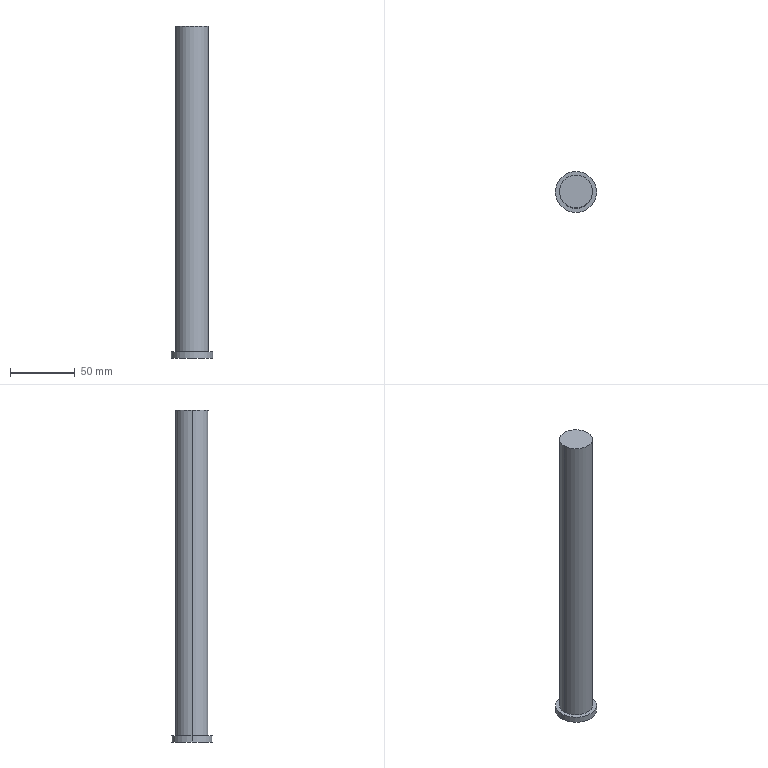Part | STEP file | 4-20.sldasm-Part-242 | 1 solid | 7 faces | box 31.75 x 31.75 x 256 mm | volume 131075 mm3 | cylinder 4 | plane 3 | commonest cylinder face diameters 25.4 x2 31.75 x2
STEP:
#1=CARTESIAN_POINT('',(105.7,-492.,-100.237));
#2=VERTEX_POINT('',#1);
#3=CARTESIAN_POINT('',(80.3,-492.,-100.237));
#4=VERTEX_POINT('',#3);
#5=CARTESIAN_POINT('',(93.,-492.,-100.237));
#6=DIRECTION('',(0.,0.,-1.));
#7=DIRECTION('',(1.,0.,0.));
#8=AXIS2_PLACEMENT_3D('',#5,#6,#7);
#9=CIRCLE('',#8,12.7);
#10=EDGE_CURVE('',#2,#4,#9,.T.);
#11=ORIENTED_EDGE('',*,*,#10,.F.);
#12=CARTESIAN_POINT('',(105.7,-492.,151.));
#13=VERTEX_POINT('',#12);
#14=CARTESIAN_POINT('',(105.7,-492.,93.299));
#15=DIRECTION('',(0.,0.,1.));
#16=VECTOR('',#15,1000.);
#17=LINE('',#14,#16);
#18=EDGE_CURVE('',#2,#13,#17,.T.);
#19=ORIENTED_EDGE('',*,*,#18,.T.);
#20=CARTESIAN_POINT('',(80.3,-492.,151.));
#21=VERTEX_POINT('',#20);
#22=CARTESIAN_POINT('',(93.,-492.,151.));
#23=DIRECTION('',(0.,0.,-1.));
#24=DIRECTION('',(1.,0.,0.));
#25=AXIS2_PLACEMENT_3D('',#22,#23,#24);
#26=CIRCLE('',#25,12.7);
#27=EDGE_CURVE('',#13,#21,#26,.T.);
#28=ORIENTED_EDGE('',*,*,#27,.T.);
#29=CARTESIAN_POINT('',(80.3,-492.,93.299));
#30=DIRECTION('',(0.,0.,1.));
#31=VECTOR('',#30,1000.);
#32=LINE('',#29,#31);
#33=EDGE_CURVE('',#4,#21,#32,.T.);
#34=ORIENTED_EDGE('',*,*,#33,.F.);
#35=EDGE_LOOP('',(#11,#19,#28,#34));
#36=FACE_OUTER_BOUND('',#35,.T.);
#37=CARTESIAN_POINT('',(93.,-492.,93.299));
#38=DIRECTION('',(0.,0.,1.));
#39=DIRECTION('',(-1.,0.,0.));
#40=AXIS2_PLACEMENT_3D('',#37,#38,#39);
#41=CYLINDRICAL_SURFACE('',#40,12.7);
#42=ADVANCED_FACE('',(#36),#41,.T.);
#43=CARTESIAN_POINT('',(108.875,-492.,-105.));
#44=VERTEX_POINT('',#43);
#45=CARTESIAN_POINT('',(77.125,-492.,-105.));
#46=VERTEX_POINT('',#45);
#47=CARTESIAN_POINT('',(93.,-492.,-105.));
#48=DIRECTION('',(0.,0.,-1.));
#49=DIRECTION('',(1.,0.,0.));
#50=AXIS2_PLACEMENT_3D('',#47,#48,#49);
#51=CIRCLE('',#50,15.875);
#52=EDGE_CURVE('',#44,#46,#51,.T.);
#53=ORIENTED_EDGE('',*,*,#52,.F.);
#54=CARTESIAN_POINT('',(108.875,-492.,-100.237));
#55=VERTEX_POINT('',#54);
#56=CARTESIAN_POINT('',(108.875,-492.,93.299));
#57=DIRECTION('',(0.,0.,1.));
#58=VECTOR('',#57,1000.);
#59=LINE('',#56,#58);
#60=EDGE_CURVE('',#44,#55,#59,.T.);
#61=ORIENTED_EDGE('',*,*,#60,.T.);
#62=CARTESIAN_POINT('',(77.125,-492.,-100.237));
#63=VERTEX_POINT('',#62);
#64=CARTESIAN_POINT('',(93.,-492.,-100.237));
#65=DIRECTION('',(0.,0.,-1.));
#66=DIRECTION('',(1.,0.,0.));
#67=AXIS2_PLACEMENT_3D('',#64,#65,#66);
#68=CIRCLE('',#67,15.875);
#69=EDGE_CURVE('',#55,#63,#68,.T.);
#70=ORIENTED_EDGE('',*,*,#69,.T.);
#71=CARTESIAN_POINT('',(77.125,-492.,93.299));
#72=DIRECTION('',(0.,0.,1.));
#73=VECTOR('',#72,1000.);
#74=LINE('',#71,#73);
#75=EDGE_CURVE('',#46,#63,#74,.T.);
#76=ORIENTED_EDGE('',*,*,#75,.F.);
#77=EDGE_LOOP('',(#53,#61,#70,#76));
#78=FACE_OUTER_BOUND('',#77,.T.);
#79=CARTESIAN_POINT('',(93.,-492.,93.299));
#80=DIRECTION('',(0.,0.,1.));
#81=DIRECTION('',(-1.,0.,0.));
#82=AXIS2_PLACEMENT_3D('',#79,#80,#81);
#83=CYLINDRICAL_SURFACE('',#82,15.875);
#84=ADVANCED_FACE('',(#78),#83,.T.);
#85=CARTESIAN_POINT('',(93.,-492.,-100.237));
#86=DIRECTION('',(0.,0.,-1.));
#87=DIRECTION('',(1.,0.,0.));
#88=AXIS2_PLACEMENT_3D('',#85,#86,#87);
#89=CIRCLE('',#88,12.7);
#90=EDGE_CURVE('',#4,#2,#89,.T.);
#91=ORIENTED_EDGE('',*,*,#90,.T.);
#92=ORIENTED_EDGE('',*,*,#10,.T.);
#93=EDGE_LOOP('',(#91,#92));
#94=FACE_BOUND('',#93,.T.);
#95=CARTESIAN_POINT('',(93.,-492.,-100.237));
#96=DIRECTION('',(0.,0.,-1.));
#97=DIRECTION('',(1.,0.,0.));
#98=AXIS2_PLACEMENT_3D('',#95,#96,#97);
#99=CIRCLE('',#98,15.875);
#100=EDGE_CURVE('',#63,#55,#99,.T.);
#101=ORIENTED_EDGE('',*,*,#100,.F.);
#102=ORIENTED_EDGE('',*,*,#69,.F.);
#103=EDGE_LOOP('',(#101,#102));
#104=FACE_OUTER_BOUND('',#103,.T.);
#105=CARTESIAN_POINT('',(93.,-492.,-100.237));
#106=DIRECTION('',(0.,0.,1.));
#107=DIRECTION('',(-1.,0.,0.));
#108=AXIS2_PLACEMENT_3D('',#105,#106,#107);
#109=PLANE('',#108);
#110=ADVANCED_FACE('',(#94,#104),#109,.T.);
#111=CARTESIAN_POINT('',(93.,-492.,-105.));
#112=DIRECTION('',(0.,0.,-1.));
#113=DIRECTION('',(1.,0.,0.));
#114=AXIS2_PLACEMENT_3D('',#111,#112,#113);
#115=CIRCLE('',#114,15.875);
#116=EDGE_CURVE('',#46,#44,#115,.T.);
#117=ORIENTED_EDGE('',*,*,#116,.T.);
#118=ORIENTED_EDGE('',*,*,#52,.T.);
#119=EDGE_LOOP('',(#117,#118));
#120=FACE_OUTER_BOUND('',#119,.T.);
#121=CARTESIAN_POINT('',(93.,-492.,-105.));
#122=DIRECTION('',(0.,0.,1.));
#123=DIRECTION('',(-1.,0.,0.));
#124=AXIS2_PLACEMENT_3D('',#121,#122,#123);
#125=PLANE('',#124);
#126=ADVANCED_FACE('',(#120),#125,.F.);
#127=ORIENTED_EDGE('',*,*,#60,.F.);
#128=ORIENTED_EDGE('',*,*,#116,.F.);
#129=ORIENTED_EDGE('',*,*,#75,.T.);
#130=ORIENTED_EDGE('',*,*,#100,.T.);
#131=EDGE_LOOP('',(#127,#128,#129,#130));
#132=FACE_OUTER_BOUND('',#131,.T.);
#133=CARTESIAN_POINT('',(93.,-492.,93.299));
#134=DIRECTION('',(0.,0.,1.));
#135=DIRECTION('',(-1.,0.,0.));
#136=AXIS2_PLACEMENT_3D('',#133,#134,#135);
#137=CYLINDRICAL_SURFACE('',#136,15.875);
#138=ADVANCED_FACE('',(#132),#137,.T.);
#139=CARTESIAN_POINT('',(93.,-492.,151.));
#140=DIRECTION('',(0.,0.,-1.));
#141=DIRECTION('',(1.,0.,0.));
#142=AXIS2_PLACEMENT_3D('',#139,#140,#141);
#143=CIRCLE('',#142,12.7);
#144=EDGE_CURVE('',#21,#13,#143,.T.);
#145=ORIENTED_EDGE('',*,*,#144,.F.);
#146=ORIENTED_EDGE('',*,*,#27,.F.);
#147=EDGE_LOOP('',(#145,#146));
#148=FACE_OUTER_BOUND('',#147,.T.);
#149=CARTESIAN_POINT('',(80.,0.,151.));
#150=DIRECTION('',(0.,0.,-1.));
#151=DIRECTION('',(1.,0.,0.));
#152=AXIS2_PLACEMENT_3D('',#149,#150,#151);
#153=PLANE('',#152);
#154=ADVANCED_FACE('',(#148),#153,.F.);
#155=ORIENTED_EDGE('',*,*,#18,.F.);
#156=ORIENTED_EDGE('',*,*,#90,.F.);
#157=ORIENTED_EDGE('',*,*,#33,.T.);
#158=ORIENTED_EDGE('',*,*,#144,.T.);
#159=EDGE_LOOP('',(#155,#156,#157,#158));
#160=FACE_OUTER_BOUND('',#159,.T.);
#161=CARTESIAN_POINT('',(93.,-492.,93.299));
#162=DIRECTION('',(0.,0.,1.));
#163=DIRECTION('',(-1.,0.,0.));
#164=AXIS2_PLACEMENT_3D('',#161,#162,#163);
#165=CYLINDRICAL_SURFACE('',#164,12.7);
#166=ADVANCED_FACE('',(#160),#165,.T.);
#167=CLOSED_SHELL('',(#42,#84,#110,#126,#138,#154,#166));
#168=MANIFOLD_SOLID_BREP('',#167);
#169=CARTESIAN_POINT('',(0.,0.,0.));
#170=DIRECTION('',(0.,0.,1.));
#171=DIRECTION('',(1.,0.,0.));
#172=AXIS2_PLACEMENT_3D('',#169,#170,#171);
#173=(LENGTH_UNIT()NAMED_UNIT(*)SI_UNIT(.MILLI.,.METRE.));
#174=UNCERTAINTY_MEASURE_WITH_UNIT(LENGTH_MEASURE(0.00001),#173,'','');
#175=(NAMED_UNIT(*)PLANE_ANGLE_UNIT()SI_UNIT($,.RADIAN.));
#176=(NAMED_UNIT(*)SI_UNIT($,.STERADIAN.)SOLID_ANGLE_UNIT());
#177=(GEOMETRIC_REPRESENTATION_CONTEXT(3)GLOBAL_UNCERTAINTY_ASSIGNED_CONTEXT((#174))GLOBAL_UNIT_ASSIGNED_CONTEXT((#173,#175,#176))REPRESENTATION_CONTEXT('',''));
#178=ADVANCED_BREP_SHAPE_REPRESENTATION('',(#168,#172),#177);